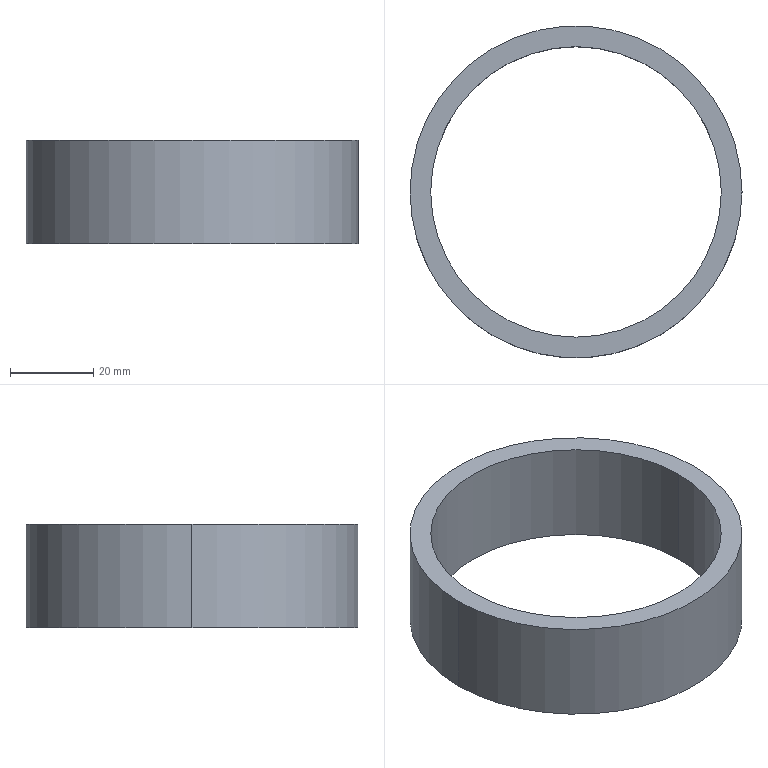Part | SolidWorks | features Extrusion 1 | 1 solid | 6 faces | box 80 x 80 x 25 mm | volume 29452 mm3 | cylinder 4 | plane 2 | commonest cylinder face diameters 70 x2 80 x2
STEP:
#1=CARTESIAN_POINT('',(-35.,0.,-12.5));
#2=VERTEX_POINT('',#1);
#3=CARTESIAN_POINT('',(35.,0.,-12.5));
#4=VERTEX_POINT('',#3);
#5=CARTESIAN_POINT('',(0.,0.,-12.5));
#6=DIRECTION('',(0.,0.,1.));
#7=DIRECTION('',(1.,0.,0.));
#8=AXIS2_PLACEMENT_3D('',#5,#6,#7);
#9=CIRCLE('',#8,35.);
#10=EDGE_CURVE('',#2,#4,#9,.T.);
#11=ORIENTED_EDGE('',*,*,#10,.F.);
#12=CARTESIAN_POINT('',(-35.,0.,12.5));
#13=VERTEX_POINT('',#12);
#14=CARTESIAN_POINT('',(-35.,0.,-12.5));
#15=DIRECTION('',(0.,0.,1.));
#16=VECTOR('',#15,1000.);
#17=LINE('',#14,#16);
#18=EDGE_CURVE('',#2,#13,#17,.T.);
#19=ORIENTED_EDGE('',*,*,#18,.T.);
#20=CARTESIAN_POINT('',(35.,0.,12.5));
#21=VERTEX_POINT('',#20);
#22=CARTESIAN_POINT('',(0.,0.,12.5));
#23=DIRECTION('',(0.,0.,1.));
#24=DIRECTION('',(1.,0.,0.));
#25=AXIS2_PLACEMENT_3D('',#22,#23,#24);
#26=CIRCLE('',#25,35.);
#27=EDGE_CURVE('',#13,#21,#26,.T.);
#28=ORIENTED_EDGE('',*,*,#27,.T.);
#29=CARTESIAN_POINT('',(35.,0.,-12.5));
#30=DIRECTION('',(0.,0.,1.));
#31=VECTOR('',#30,1000.);
#32=LINE('',#29,#31);
#33=EDGE_CURVE('',#4,#21,#32,.T.);
#34=ORIENTED_EDGE('',*,*,#33,.F.);
#35=EDGE_LOOP('',(#11,#19,#28,#34));
#36=FACE_OUTER_BOUND('',#35,.T.);
#37=CARTESIAN_POINT('',(0.,0.,-12.5));
#38=DIRECTION('',(0.,0.,1.));
#39=DIRECTION('',(1.,0.,0.));
#40=AXIS2_PLACEMENT_3D('',#37,#38,#39);
#41=CYLINDRICAL_SURFACE('',#40,35.);
#42=ADVANCED_FACE('',(#36),#41,.F.);
#43=CARTESIAN_POINT('',(40.,0.,-12.5));
#44=VERTEX_POINT('',#43);
#45=CARTESIAN_POINT('',(-40.,0.,-12.5));
#46=VERTEX_POINT('',#45);
#47=CARTESIAN_POINT('',(0.,0.,-12.5));
#48=DIRECTION('',(0.,0.,1.));
#49=DIRECTION('',(1.,0.,0.));
#50=AXIS2_PLACEMENT_3D('',#47,#48,#49);
#51=CIRCLE('',#50,40.);
#52=EDGE_CURVE('',#44,#46,#51,.T.);
#53=ORIENTED_EDGE('',*,*,#52,.T.);
#54=CARTESIAN_POINT('',(-40.,0.,12.5));
#55=VERTEX_POINT('',#54);
#56=CARTESIAN_POINT('',(-40.,0.,-12.5));
#57=DIRECTION('',(0.,0.,1.));
#58=VECTOR('',#57,1000.);
#59=LINE('',#56,#58);
#60=EDGE_CURVE('',#46,#55,#59,.T.);
#61=ORIENTED_EDGE('',*,*,#60,.T.);
#62=CARTESIAN_POINT('',(40.,0.,12.5));
#63=VERTEX_POINT('',#62);
#64=CARTESIAN_POINT('',(0.,0.,12.5));
#65=DIRECTION('',(0.,0.,1.));
#66=DIRECTION('',(1.,0.,0.));
#67=AXIS2_PLACEMENT_3D('',#64,#65,#66);
#68=CIRCLE('',#67,40.);
#69=EDGE_CURVE('',#63,#55,#68,.T.);
#70=ORIENTED_EDGE('',*,*,#69,.F.);
#71=CARTESIAN_POINT('',(40.,0.,-12.5));
#72=DIRECTION('',(0.,0.,1.));
#73=VECTOR('',#72,1000.);
#74=LINE('',#71,#73);
#75=EDGE_CURVE('',#44,#63,#74,.T.);
#76=ORIENTED_EDGE('',*,*,#75,.F.);
#77=EDGE_LOOP('',(#53,#61,#70,#76));
#78=FACE_OUTER_BOUND('',#77,.T.);
#79=CARTESIAN_POINT('',(0.,0.,-12.5));
#80=DIRECTION('',(0.,0.,1.));
#81=DIRECTION('',(1.,0.,0.));
#82=AXIS2_PLACEMENT_3D('',#79,#80,#81);
#83=CYLINDRICAL_SURFACE('',#82,40.);
#84=ADVANCED_FACE('',(#78),#83,.T.);
#85=ORIENTED_EDGE('',*,*,#60,.F.);
#86=CARTESIAN_POINT('',(0.,0.,-12.5));
#87=DIRECTION('',(0.,0.,1.));
#88=DIRECTION('',(1.,0.,0.));
#89=AXIS2_PLACEMENT_3D('',#86,#87,#88);
#90=CIRCLE('',#89,40.);
#91=EDGE_CURVE('',#46,#44,#90,.T.);
#92=ORIENTED_EDGE('',*,*,#91,.T.);
#93=ORIENTED_EDGE('',*,*,#75,.T.);
#94=CARTESIAN_POINT('',(0.,0.,12.5));
#95=DIRECTION('',(0.,0.,1.));
#96=DIRECTION('',(1.,0.,0.));
#97=AXIS2_PLACEMENT_3D('',#94,#95,#96);
#98=CIRCLE('',#97,40.);
#99=EDGE_CURVE('',#55,#63,#98,.T.);
#100=ORIENTED_EDGE('',*,*,#99,.F.);
#101=EDGE_LOOP('',(#85,#92,#93,#100));
#102=FACE_OUTER_BOUND('',#101,.T.);
#103=CARTESIAN_POINT('',(0.,0.,-12.5));
#104=DIRECTION('',(0.,0.,1.));
#105=DIRECTION('',(1.,0.,0.));
#106=AXIS2_PLACEMENT_3D('',#103,#104,#105);
#107=CYLINDRICAL_SURFACE('',#106,40.);
#108=ADVANCED_FACE('',(#102),#107,.T.);
#109=CARTESIAN_POINT('',(0.,0.,-12.5));
#110=DIRECTION('',(0.,0.,1.));
#111=DIRECTION('',(1.,0.,0.));
#112=AXIS2_PLACEMENT_3D('',#109,#110,#111);
#113=CIRCLE('',#112,35.);
#114=EDGE_CURVE('',#4,#2,#113,.T.);
#115=ORIENTED_EDGE('',*,*,#114,.T.);
#116=ORIENTED_EDGE('',*,*,#10,.T.);
#117=EDGE_LOOP('',(#115,#116));
#118=FACE_BOUND('',#117,.T.);
#119=ORIENTED_EDGE('',*,*,#52,.F.);
#120=ORIENTED_EDGE('',*,*,#91,.F.);
#121=EDGE_LOOP('',(#119,#120));
#122=FACE_OUTER_BOUND('',#121,.T.);
#123=CARTESIAN_POINT('',(0.,0.,-12.5));
#124=DIRECTION('',(0.,0.,1.));
#125=DIRECTION('',(1.,0.,0.));
#126=AXIS2_PLACEMENT_3D('',#123,#124,#125);
#127=PLANE('',#126);
#128=ADVANCED_FACE('',(#118,#122),#127,.F.);
#129=CARTESIAN_POINT('',(0.,0.,12.5));
#130=DIRECTION('',(0.,0.,1.));
#131=DIRECTION('',(1.,0.,0.));
#132=AXIS2_PLACEMENT_3D('',#129,#130,#131);
#133=CIRCLE('',#132,35.);
#134=EDGE_CURVE('',#21,#13,#133,.T.);
#135=ORIENTED_EDGE('',*,*,#134,.F.);
#136=ORIENTED_EDGE('',*,*,#27,.F.);
#137=EDGE_LOOP('',(#135,#136));
#138=FACE_BOUND('',#137,.T.);
#139=ORIENTED_EDGE('',*,*,#69,.T.);
#140=ORIENTED_EDGE('',*,*,#99,.T.);
#141=EDGE_LOOP('',(#139,#140));
#142=FACE_OUTER_BOUND('',#141,.T.);
#143=CARTESIAN_POINT('',(0.,0.,12.5));
#144=DIRECTION('',(0.,0.,1.));
#145=DIRECTION('',(1.,0.,0.));
#146=AXIS2_PLACEMENT_3D('',#143,#144,#145);
#147=PLANE('',#146);
#148=ADVANCED_FACE('',(#138,#142),#147,.T.);
#149=ORIENTED_EDGE('',*,*,#18,.F.);
#150=ORIENTED_EDGE('',*,*,#114,.F.);
#151=ORIENTED_EDGE('',*,*,#33,.T.);
#152=ORIENTED_EDGE('',*,*,#134,.T.);
#153=EDGE_LOOP('',(#149,#150,#151,#152));
#154=FACE_OUTER_BOUND('',#153,.T.);
#155=CARTESIAN_POINT('',(0.,0.,-12.5));
#156=DIRECTION('',(0.,0.,1.));
#157=DIRECTION('',(1.,0.,0.));
#158=AXIS2_PLACEMENT_3D('',#155,#156,#157);
#159=CYLINDRICAL_SURFACE('',#158,35.);
#160=ADVANCED_FACE('',(#154),#159,.F.);
#161=CLOSED_SHELL('',(#42,#84,#108,#128,#148,#160));
#162=MANIFOLD_SOLID_BREP('',#161);
#163=CARTESIAN_POINT('',(0.,0.,0.));
#164=DIRECTION('',(0.,0.,1.));
#165=DIRECTION('',(1.,0.,0.));
#166=AXIS2_PLACEMENT_3D('',#163,#164,#165);
#167=(LENGTH_UNIT()NAMED_UNIT(*)SI_UNIT(.MILLI.,.METRE.));
#168=UNCERTAINTY_MEASURE_WITH_UNIT(LENGTH_MEASURE(0.00001),#167,'','');
#169=(NAMED_UNIT(*)PLANE_ANGLE_UNIT()SI_UNIT($,.RADIAN.));
#170=(NAMED_UNIT(*)SI_UNIT($,.STERADIAN.)SOLID_ANGLE_UNIT());
#171=(GEOMETRIC_REPRESENTATION_CONTEXT(3)GLOBAL_UNCERTAINTY_ASSIGNED_CONTEXT((#168))GLOBAL_UNIT_ASSIGNED_CONTEXT((#167,#169,#170))REPRESENTATION_CONTEXT('',''));
#172=ADVANCED_BREP_SHAPE_REPRESENTATION('',(#162,#166),#171);